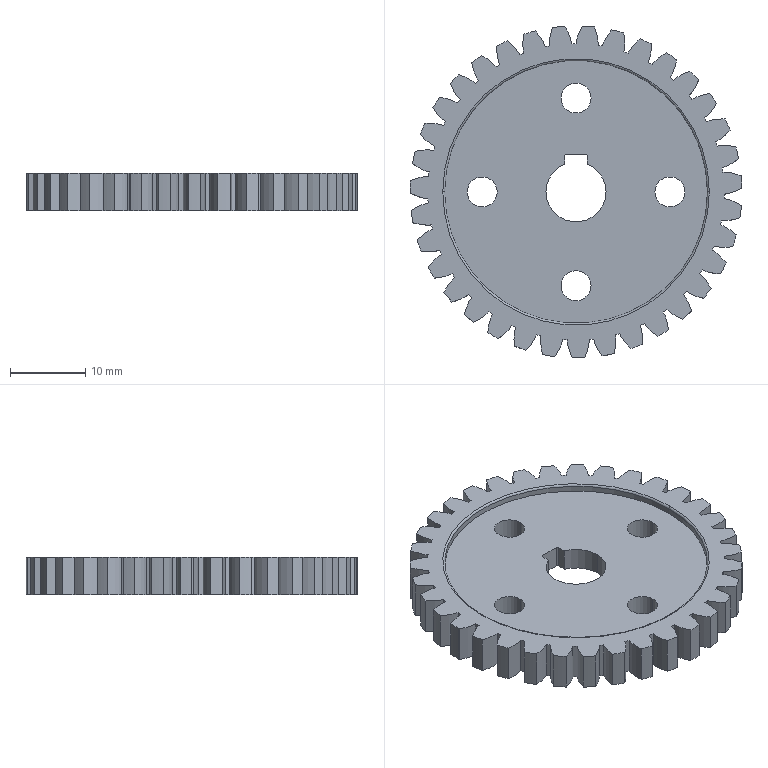Part | SolidWorks | features ICE 4, Fillet 2, Extrusion 1 | 1 solid | 169 faces | box 44.212 x 44.202 x 5 mm | volume 4910 mm3 | cylinder 88 | spline 70 | plane 7 | torus 4 | commonest cylinder face diameters 44.218 x36 39.5 x35 4 x8 35 x4 8 x3 0.4 x2